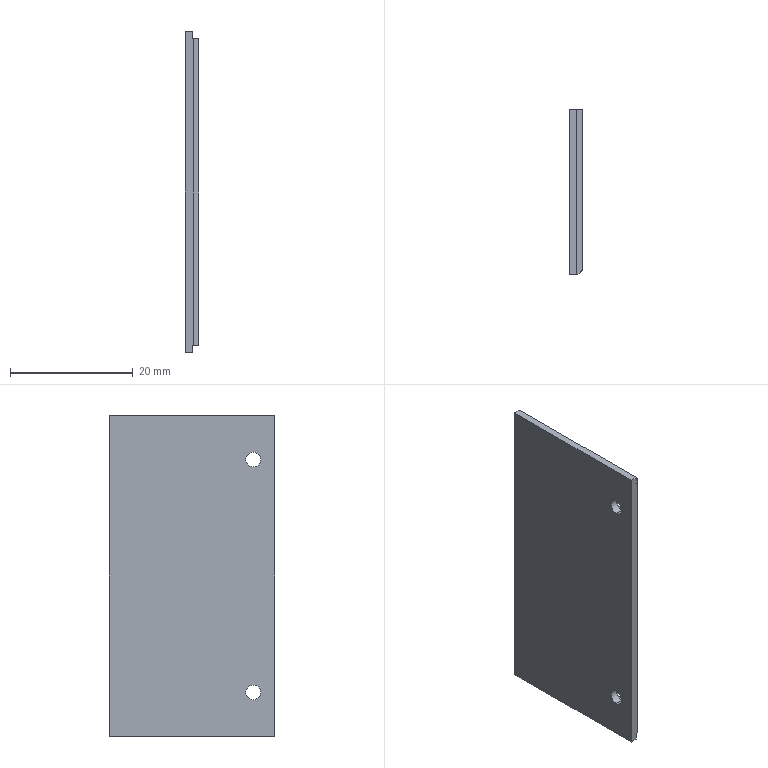Part | STEP file | ASND-0110-OPT-CO60-X-V1.0 lower cover plate | 1 solid | 19 faces | box 2.2 x 27 x 52.3 mm | volume 2996 mm3 | plane 11 | cone 4 | cylinder 4 | commonest cylinder face diameters 2.4 x4
STEP:
#1=CARTESIAN_POINT('',(0.,0.,0.));
#2=DIRECTION('',(0.,0.,1.));
#3=DIRECTION('',(1.,0.,0.));
#4=AXIS2_PLACEMENT_3D('',#1,#2,#3);
#5=CARTESIAN_POINT('',(1.2,-10.,17.8));
#6=VERTEX_POINT('',#5);
#7=CARTESIAN_POINT('',(2.2,-10.,16.8));
#8=VERTEX_POINT('',#7);
#9=CARTESIAN_POINT('',(1.2,-10.,17.8));
#10=DIRECTION('',(0.7071,0.,-0.7071));
#11=VECTOR('',#10,1.);
#12=LINE('',#9,#11);
#13=CARTESIAN_POINT('',(1.2,-10.,19.));
#14=DIRECTION('',(1.,0.,0.));
#15=DIRECTION('',(0.,0.,-1.));
#16=AXIS2_PLACEMENT_3D('',#13,#14,#15);
#17=CONICAL_SURFACE('',#16,1.2,0.7854);
#18=CARTESIAN_POINT('',(6.283,0.));
#19=DIRECTION('',(0.,1.));
#20=VECTOR('',#19,1.);
#21=LINE('',#18,#20);
#22=(GEOMETRIC_REPRESENTATION_CONTEXT(2)PARAMETRIC_REPRESENTATION_CONTEXT()REPRESENTATION_CONTEXT('',''));
#23=DEFINITIONAL_REPRESENTATION('',(#21),#22);
#24=PCURVE('',#17,#23);
#25=CARTESIAN_POINT('',(1.2,-10.,19.));
#26=DIRECTION('',(1.,0.,0.));
#27=DIRECTION('',(0.,0.,-1.));
#28=AXIS2_PLACEMENT_3D('',#25,#26,#27);
#29=CONICAL_SURFACE('',#28,1.2,0.7854);
#30=CARTESIAN_POINT('',(0.,0.));
#31=DIRECTION('',(0.,1.));
#32=VECTOR('',#31,1.);
#33=LINE('',#30,#32);
#34=(GEOMETRIC_REPRESENTATION_CONTEXT(2)PARAMETRIC_REPRESENTATION_CONTEXT()REPRESENTATION_CONTEXT('',''));
#35=DEFINITIONAL_REPRESENTATION('',(#33),#34);
#36=PCURVE('',#29,#35);
#37=SURFACE_CURVE('',#12,(#24,#36),.PCURVE_S1.);
#38=EDGE_CURVE('',#6,#8,#37,.T.);
#39=ORIENTED_EDGE('',*,*,#38,.T.);
#40=CARTESIAN_POINT('',(2.2,-10.,21.2));
#41=VERTEX_POINT('',#40);
#42=CARTESIAN_POINT('',(2.2,-10.,19.));
#43=DIRECTION('',(1.,0.,0.));
#44=DIRECTION('',(0.,0.,-1.));
#45=AXIS2_PLACEMENT_3D('',#42,#43,#44);
#46=CIRCLE('',#45,2.2);
#47=CARTESIAN_POINT('',(0.,1.));
#48=DIRECTION('',(1.,0.));
#49=VECTOR('',#48,1.);
#50=LINE('',#47,#49);
#51=(GEOMETRIC_REPRESENTATION_CONTEXT(2)PARAMETRIC_REPRESENTATION_CONTEXT()REPRESENTATION_CONTEXT('',''));
#52=DEFINITIONAL_REPRESENTATION('',(#50),#51);
#53=PCURVE('',#17,#52);
#54=CARTESIAN_POINT('',(2.2,-12.7,25.));
#55=DIRECTION('',(1.,0.,0.));
#56=DIRECTION('',(0.,0.7071,0.7071));
#57=AXIS2_PLACEMENT_3D('',#54,#55,#56);
#58=PLANE('',#57);
#59=CARTESIAN_POINT('',(-2.333,-6.152));
#60=DIRECTION('',(-0.7071,-0.7071));
#61=AXIS2_PLACEMENT_2D('',#59,#60);
#62=CIRCLE('',#61,2.2);
#63=(GEOMETRIC_REPRESENTATION_CONTEXT(2)PARAMETRIC_REPRESENTATION_CONTEXT()REPRESENTATION_CONTEXT('',''));
#64=DEFINITIONAL_REPRESENTATION('',(#62),#63);
#65=PCURVE('',#58,#64);
#66=SURFACE_CURVE('',#46,(#53,#65),.PCURVE_S1.);
#67=EDGE_CURVE('',#41,#8,#66,.T.);
#68=ORIENTED_EDGE('',*,*,#67,.F.);
#69=CARTESIAN_POINT('',(1.2,-10.,20.2));
#70=VERTEX_POINT('',#69);
#71=CARTESIAN_POINT('',(1.2,-10.,20.2));
#72=DIRECTION('',(0.7071,0.,0.7071));
#73=VECTOR('',#72,1.);
#74=LINE('',#71,#73);
#75=CARTESIAN_POINT('',(3.142,0.));
#76=DIRECTION('',(0.,1.));
#77=VECTOR('',#76,1.);
#78=LINE('',#75,#77);
#79=(GEOMETRIC_REPRESENTATION_CONTEXT(2)PARAMETRIC_REPRESENTATION_CONTEXT()REPRESENTATION_CONTEXT('',''));
#80=DEFINITIONAL_REPRESENTATION('',(#78),#79);
#81=PCURVE('',#17,#80);
#82=CARTESIAN_POINT('',(3.142,0.));
#83=DIRECTION('',(0.,1.));
#84=VECTOR('',#83,1.);
#85=LINE('',#82,#84);
#86=(GEOMETRIC_REPRESENTATION_CONTEXT(2)PARAMETRIC_REPRESENTATION_CONTEXT()REPRESENTATION_CONTEXT('',''));
#87=DEFINITIONAL_REPRESENTATION('',(#85),#86);
#88=PCURVE('',#29,#87);
#89=SURFACE_CURVE('',#74,(#81,#88),.PCURVE_S1.);
#90=EDGE_CURVE('',#70,#41,#89,.T.);
#91=ORIENTED_EDGE('',*,*,#90,.F.);
#92=CARTESIAN_POINT('',(1.2,-10.,19.));
#93=DIRECTION('',(-1.,0.,0.));
#94=DIRECTION('',(0.,0.,-1.));
#95=AXIS2_PLACEMENT_3D('',#92,#93,#94);
#96=CIRCLE('',#95,1.2);
#97=CARTESIAN_POINT('',(6.283,0.));
#98=DIRECTION('',(-1.,0.));
#99=VECTOR('',#98,1.);
#100=LINE('',#97,#99);
#101=(GEOMETRIC_REPRESENTATION_CONTEXT(2)PARAMETRIC_REPRESENTATION_CONTEXT()REPRESENTATION_CONTEXT('',''));
#102=DEFINITIONAL_REPRESENTATION('',(#100),#101);
#103=PCURVE('',#17,#102);
#104=CARTESIAN_POINT('',(0.,-10.,19.));
#105=DIRECTION('',(1.,0.,0.));
#106=DIRECTION('',(0.,0.,-1.));
#107=AXIS2_PLACEMENT_3D('',#104,#105,#106);
#108=CYLINDRICAL_SURFACE('',#107,1.2);
#109=CARTESIAN_POINT('',(6.283,1.2));
#110=DIRECTION('',(-1.,0.));
#111=VECTOR('',#110,1.);
#112=LINE('',#109,#111);
#113=(GEOMETRIC_REPRESENTATION_CONTEXT(2)PARAMETRIC_REPRESENTATION_CONTEXT()REPRESENTATION_CONTEXT('',''));
#114=DEFINITIONAL_REPRESENTATION('',(#112),#113);
#115=PCURVE('',#108,#114);
#116=SURFACE_CURVE('',#96,(#103,#115),.PCURVE_S1.);
#117=EDGE_CURVE('',#6,#70,#116,.T.);
#118=ORIENTED_EDGE('',*,*,#117,.F.);
#119=EDGE_LOOP('',(#39,#68,#91,#118));
#120=FACE_BOUND('',#119,.F.);
#121=ADVANCED_FACE('',(#120),#17,.F.);
#122=CARTESIAN_POINT('',(0.,-10.,17.8));
#123=VERTEX_POINT('',#122);
#124=CARTESIAN_POINT('',(0.,-10.,17.8));
#125=DIRECTION('',(1.,0.,0.));
#126=VECTOR('',#125,1.);
#127=LINE('',#124,#126);
#128=CARTESIAN_POINT('',(6.283,0.));
#129=DIRECTION('',(0.,1.));
#130=VECTOR('',#129,1.);
#131=LINE('',#128,#130);
#132=(GEOMETRIC_REPRESENTATION_CONTEXT(2)PARAMETRIC_REPRESENTATION_CONTEXT()REPRESENTATION_CONTEXT('',''));
#133=DEFINITIONAL_REPRESENTATION('',(#131),#132);
#134=PCURVE('',#108,#133);
#135=CARTESIAN_POINT('',(0.,-10.,19.));
#136=DIRECTION('',(1.,0.,0.));
#137=DIRECTION('',(0.,0.,-1.));
#138=AXIS2_PLACEMENT_3D('',#135,#136,#137);
#139=CYLINDRICAL_SURFACE('',#138,1.2);
#140=CARTESIAN_POINT('',(0.,0.));
#141=DIRECTION('',(0.,1.));
#142=VECTOR('',#141,1.);
#143=LINE('',#140,#142);
#144=(GEOMETRIC_REPRESENTATION_CONTEXT(2)PARAMETRIC_REPRESENTATION_CONTEXT()REPRESENTATION_CONTEXT('',''));
#145=DEFINITIONAL_REPRESENTATION('',(#143),#144);
#146=PCURVE('',#139,#145);
#147=SURFACE_CURVE('',#127,(#134,#146),.PCURVE_S1.);
#148=EDGE_CURVE('',#123,#6,#147,.T.);
#149=ORIENTED_EDGE('',*,*,#148,.T.);
#150=ORIENTED_EDGE('',*,*,#117,.T.);
#151=CARTESIAN_POINT('',(0.,-10.,20.2));
#152=VERTEX_POINT('',#151);
#153=CARTESIAN_POINT('',(0.,-10.,20.2));
#154=DIRECTION('',(1.,0.,0.));
#155=VECTOR('',#154,1.);
#156=LINE('',#153,#155);
#157=CARTESIAN_POINT('',(3.142,0.));
#158=DIRECTION('',(0.,1.));
#159=VECTOR('',#158,1.);
#160=LINE('',#157,#159);
#161=(GEOMETRIC_REPRESENTATION_CONTEXT(2)PARAMETRIC_REPRESENTATION_CONTEXT()REPRESENTATION_CONTEXT('',''));
#162=DEFINITIONAL_REPRESENTATION('',(#160),#161);
#163=PCURVE('',#108,#162);
#164=CARTESIAN_POINT('',(3.142,0.));
#165=DIRECTION('',(0.,1.));
#166=VECTOR('',#165,1.);
#167=LINE('',#164,#166);
#168=(GEOMETRIC_REPRESENTATION_CONTEXT(2)PARAMETRIC_REPRESENTATION_CONTEXT()REPRESENTATION_CONTEXT('',''));
#169=DEFINITIONAL_REPRESENTATION('',(#167),#168);
#170=PCURVE('',#139,#169);
#171=SURFACE_CURVE('',#156,(#163,#170),.PCURVE_S1.);
#172=EDGE_CURVE('',#152,#70,#171,.T.);
#173=ORIENTED_EDGE('',*,*,#172,.F.);
#174=CARTESIAN_POINT('',(0.,-10.,19.));
#175=DIRECTION('',(-1.,0.,0.));
#176=DIRECTION('',(0.,0.,-1.));
#177=AXIS2_PLACEMENT_3D('',#174,#175,#176);
#178=CIRCLE('',#177,1.2);
#179=CARTESIAN_POINT('',(6.283,0.));
#180=DIRECTION('',(-1.,0.));
#181=VECTOR('',#180,1.);
#182=LINE('',#179,#181);
#183=(GEOMETRIC_REPRESENTATION_CONTEXT(2)PARAMETRIC_REPRESENTATION_CONTEXT()REPRESENTATION_CONTEXT('',''));
#184=DEFINITIONAL_REPRESENTATION('',(#182),#183);
#185=PCURVE('',#108,#184);
#186=CARTESIAN_POINT('',(0.,-13.5,26.15));
#187=DIRECTION('',(1.,0.,0.));
#188=DIRECTION('',(0.,0.7071,0.7071));
#189=AXIS2_PLACEMENT_3D('',#186,#187,#188);
#190=PLANE('',#189);
#191=CARTESIAN_POINT('',(-3.429,-8.379));
#192=CARTESIAN_POINT('',(-4.899,-6.91));
#193=CARTESIAN_POINT('',(-2.892,-6.372));
#194=CARTESIAN_POINT('',(-0.8839,-5.834));
#195=CARTESIAN_POINT('',(-1.422,-7.841));
#196=CARTESIAN_POINT('',(-1.96,-9.849));
#197=CARTESIAN_POINT('',(-3.429,-8.379));
#198=(BOUNDED_CURVE()B_SPLINE_CURVE(2,(#191,#192,#193,#194,#195,#196,#197),.UNSPECIFIED.,.T.,.F.)B_SPLINE_CURVE_WITH_KNOTS((1,2,2,2,2,1),(-2.094,0.,2.094,4.189,6.283,8.378),.UNSPECIFIED.)CURVE()GEOMETRIC_REPRESENTATION_ITEM()RATIONAL_B_SPLINE_CURVE((1.,0.5,1.,0.5,1.,0.5,1.))REPRESENTATION_ITEM(''));
#199=(GEOMETRIC_REPRESENTATION_CONTEXT(2)PARAMETRIC_REPRESENTATION_CONTEXT()REPRESENTATION_CONTEXT('',''));
#200=DEFINITIONAL_REPRESENTATION('',(#198),#199);
#201=PCURVE('',#190,#200);
#202=SURFACE_CURVE('',#178,(#185,#201),.PCURVE_S1.);
#203=EDGE_CURVE('',#123,#152,#202,.T.);
#204=ORIENTED_EDGE('',*,*,#203,.F.);
#205=EDGE_LOOP('',(#149,#150,#173,#204));
#206=FACE_BOUND('',#205,.F.);
#207=ADVANCED_FACE('',(#206),#108,.F.);
#208=CARTESIAN_POINT('',(1.2,-10.,-20.2));
#209=VERTEX_POINT('',#208);
#210=CARTESIAN_POINT('',(2.2,-10.,-21.2));
#211=VERTEX_POINT('',#210);
#212=CARTESIAN_POINT('',(1.2,-10.,-20.2));
#213=DIRECTION('',(0.7071,0.,-0.7071));
#214=VECTOR('',#213,1.);
#215=LINE('',#212,#214);
#216=CARTESIAN_POINT('',(1.2,-10.,-19.));
#217=DIRECTION('',(1.,0.,0.));
#218=DIRECTION('',(0.,0.,-1.));
#219=AXIS2_PLACEMENT_3D('',#216,#217,#218);
#220=CONICAL_SURFACE('',#219,1.2,0.7854);
#221=CARTESIAN_POINT('',(6.283,0.));
#222=DIRECTION('',(0.,1.));
#223=VECTOR('',#222,1.);
#224=LINE('',#221,#223);
#225=(GEOMETRIC_REPRESENTATION_CONTEXT(2)PARAMETRIC_REPRESENTATION_CONTEXT()REPRESENTATION_CONTEXT('',''));
#226=DEFINITIONAL_REPRESENTATION('',(#224),#225);
#227=PCURVE('',#220,#226);
#228=CARTESIAN_POINT('',(1.2,-10.,-19.));
#229=DIRECTION('',(1.,0.,0.));
#230=DIRECTION('',(0.,0.,-1.));
#231=AXIS2_PLACEMENT_3D('',#228,#229,#230);
#232=CONICAL_SURFACE('',#231,1.2,0.7854);
#233=CARTESIAN_POINT('',(0.,0.));
#234=DIRECTION('',(0.,1.));
#235=VECTOR('',#234,1.);
#236=LINE('',#233,#235);
#237=(GEOMETRIC_REPRESENTATION_CONTEXT(2)PARAMETRIC_REPRESENTATION_CONTEXT()REPRESENTATION_CONTEXT('',''));
#238=DEFINITIONAL_REPRESENTATION('',(#236),#237);
#239=PCURVE('',#232,#238);
#240=SURFACE_CURVE('',#215,(#227,#239),.PCURVE_S1.);
#241=EDGE_CURVE('',#209,#211,#240,.T.);
#242=ORIENTED_EDGE('',*,*,#241,.T.);
#243=CARTESIAN_POINT('',(2.2,-10.,-16.8));
#244=VERTEX_POINT('',#243);
#245=CARTESIAN_POINT('',(2.2,-10.,-19.));
#246=DIRECTION('',(-1.,0.,0.));
#247=DIRECTION('',(0.,0.,-1.));
#248=AXIS2_PLACEMENT_3D('',#245,#246,#247);
#249=CIRCLE('',#248,2.2);
#250=CARTESIAN_POINT('',(6.283,1.));
#251=DIRECTION('',(-1.,0.));
#252=VECTOR('',#251,1.);
#253=LINE('',#250,#252);
#254=(GEOMETRIC_REPRESENTATION_CONTEXT(2)PARAMETRIC_REPRESENTATION_CONTEXT()REPRESENTATION_CONTEXT('',''));
#255=DEFINITIONAL_REPRESENTATION('',(#253),#254);
#256=PCURVE('',#220,#255);
#257=CARTESIAN_POINT('',(-30.759,-34.578));
#258=CARTESIAN_POINT('',(-33.454,-31.883));
#259=CARTESIAN_POINT('',(-29.773,-30.897));
#260=CARTESIAN_POINT('',(-26.092,-29.911));
#261=CARTESIAN_POINT('',(-27.078,-33.591));
#262=CARTESIAN_POINT('',(-28.065,-37.272));
#263=CARTESIAN_POINT('',(-30.759,-34.578));
#264=(BOUNDED_CURVE()B_SPLINE_CURVE(2,(#257,#258,#259,#260,#261,#262,#263),.UNSPECIFIED.,.T.,.F.)B_SPLINE_CURVE_WITH_KNOTS((1,2,2,2,2,1),(-2.094,0.,2.094,4.189,6.283,8.378),.UNSPECIFIED.)CURVE()GEOMETRIC_REPRESENTATION_ITEM()RATIONAL_B_SPLINE_CURVE((1.,0.5,1.,0.5,1.,0.5,1.))REPRESENTATION_ITEM(''));
#265=(GEOMETRIC_REPRESENTATION_CONTEXT(2)PARAMETRIC_REPRESENTATION_CONTEXT()REPRESENTATION_CONTEXT('',''));
#266=DEFINITIONAL_REPRESENTATION('',(#264),#265);
#267=PCURVE('',#58,#266);
#268=SURFACE_CURVE('',#249,(#256,#267),.PCURVE_S1.);
#269=EDGE_CURVE('',#211,#244,#268,.T.);
#270=ORIENTED_EDGE('',*,*,#269,.T.);
#271=CARTESIAN_POINT('',(1.2,-10.,-17.8));
#272=VERTEX_POINT('',#271);
#273=CARTESIAN_POINT('',(1.2,-10.,-17.8));
#274=DIRECTION('',(0.7071,0.,0.7071));
#275=VECTOR('',#274,1.);
#276=LINE('',#273,#275);
#277=CARTESIAN_POINT('',(3.142,0.));
#278=DIRECTION('',(0.,1.));
#279=VECTOR('',#278,1.);
#280=LINE('',#277,#279);
#281=(GEOMETRIC_REPRESENTATION_CONTEXT(2)PARAMETRIC_REPRESENTATION_CONTEXT()REPRESENTATION_CONTEXT('',''));
#282=DEFINITIONAL_REPRESENTATION('',(#280),#281);
#283=PCURVE('',#220,#282);
#284=CARTESIAN_POINT('',(3.142,0.));
#285=DIRECTION('',(0.,1.));
#286=VECTOR('',#285,1.);
#287=LINE('',#284,#286);
#288=(GEOMETRIC_REPRESENTATION_CONTEXT(2)PARAMETRIC_REPRESENTATION_CONTEXT()REPRESENTATION_CONTEXT('',''));
#289=DEFINITIONAL_REPRESENTATION('',(#287),#288);
#290=PCURVE('',#232,#289);
#291=SURFACE_CURVE('',#276,(#283,#290),.PCURVE_S1.);
#292=EDGE_CURVE('',#272,#244,#291,.T.);
#293=ORIENTED_EDGE('',*,*,#292,.F.);
#294=CARTESIAN_POINT('',(1.2,-10.,-19.));
#295=DIRECTION('',(-1.,0.,0.));
#296=DIRECTION('',(0.,0.,-1.));
#297=AXIS2_PLACEMENT_3D('',#294,#295,#296);
#298=CIRCLE('',#297,1.2);
#299=CARTESIAN_POINT('',(6.283,0.));
#300=DIRECTION('',(-1.,0.));
#301=VECTOR('',#300,1.);
#302=LINE('',#299,#301);
#303=(GEOMETRIC_REPRESENTATION_CONTEXT(2)PARAMETRIC_REPRESENTATION_CONTEXT()REPRESENTATION_CONTEXT('',''));
#304=DEFINITIONAL_REPRESENTATION('',(#302),#303);
#305=PCURVE('',#220,#304);
#306=CARTESIAN_POINT('',(0.,-10.,-19.));
#307=DIRECTION('',(1.,0.,0.));
#308=DIRECTION('',(0.,0.,-1.));
#309=AXIS2_PLACEMENT_3D('',#306,#307,#308);
#310=CYLINDRICAL_SURFACE('',#309,1.2);
#311=CARTESIAN_POINT('',(6.283,1.2));
#312=DIRECTION('',(-1.,0.));
#313=VECTOR('',#312,1.);
#314=LINE('',#311,#313);
#315=(GEOMETRIC_REPRESENTATION_CONTEXT(2)PARAMETRIC_REPRESENTATION_CONTEXT()REPRESENTATION_CONTEXT('',''));
#316=DEFINITIONAL_REPRESENTATION('',(#314),#315);
#317=PCURVE('',#310,#316);
#318=SURFACE_CURVE('',#298,(#305,#317),.PCURVE_S1.);
#319=EDGE_CURVE('',#209,#272,#318,.T.);
#320=ORIENTED_EDGE('',*,*,#319,.F.);
#321=EDGE_LOOP('',(#242,#270,#293,#320));
#322=FACE_BOUND('',#321,.F.);
#323=ADVANCED_FACE('',(#322),#220,.F.);
#324=CARTESIAN_POINT('',(0.,-10.,-20.2));
#325=VERTEX_POINT('',#324);
#326=CARTESIAN_POINT('',(0.,-10.,-20.2));
#327=DIRECTION('',(1.,0.,0.));
#328=VECTOR('',#327,1.);
#329=LINE('',#326,#328);
#330=CARTESIAN_POINT('',(6.283,0.));
#331=DIRECTION('',(0.,1.));
#332=VECTOR('',#331,1.);
#333=LINE('',#330,#332);
#334=(GEOMETRIC_REPRESENTATION_CONTEXT(2)PARAMETRIC_REPRESENTATION_CONTEXT()REPRESENTATION_CONTEXT('',''));
#335=DEFINITIONAL_REPRESENTATION('',(#333),#334);
#336=PCURVE('',#310,#335);
#337=CARTESIAN_POINT('',(0.,-10.,-19.));
#338=DIRECTION('',(1.,0.,0.));
#339=DIRECTION('',(0.,0.,-1.));
#340=AXIS2_PLACEMENT_3D('',#337,#338,#339);
#341=CYLINDRICAL_SURFACE('',#340,1.2);
#342=CARTESIAN_POINT('',(0.,0.));
#343=DIRECTION('',(0.,1.));
#344=VECTOR('',#343,1.);
#345=LINE('',#342,#344);
#346=(GEOMETRIC_REPRESENTATION_CONTEXT(2)PARAMETRIC_REPRESENTATION_CONTEXT()REPRESENTATION_CONTEXT('',''));
#347=DEFINITIONAL_REPRESENTATION('',(#345),#346);
#348=PCURVE('',#341,#347);
#349=SURFACE_CURVE('',#329,(#336,#348),.PCURVE_S1.);
#350=EDGE_CURVE('',#325,#209,#349,.T.);
#351=ORIENTED_EDGE('',*,*,#350,.T.);
#352=ORIENTED_EDGE('',*,*,#319,.T.);
#353=CARTESIAN_POINT('',(0.,-10.,-17.8));
#354=VERTEX_POINT('',#353);
#355=CARTESIAN_POINT('',(0.,-10.,-17.8));
#356=DIRECTION('',(1.,0.,0.));
#357=VECTOR('',#356,1.);
#358=LINE('',#355,#357);
#359=CARTESIAN_POINT('',(3.142,0.));
#360=DIRECTION('',(0.,1.));
#361=VECTOR('',#360,1.);
#362=LINE('',#359,#361);
#363=(GEOMETRIC_REPRESENTATION_CONTEXT(2)PARAMETRIC_REPRESENTATION_CONTEXT()REPRESENTATION_CONTEXT('',''));
#364=DEFINITIONAL_REPRESENTATION('',(#362),#363);
#365=PCURVE('',#310,#364);
#366=CARTESIAN_POINT('',(3.142,0.));
#367=DIRECTION('',(0.,1.));
#368=VECTOR('',#367,1.);
#369=LINE('',#366,#368);
#370=(GEOMETRIC_REPRESENTATION_CONTEXT(2)PARAMETRIC_REPRESENTATION_CONTEXT()REPRESENTATION_CONTEXT('',''));
#371=DEFINITIONAL_REPRESENTATION('',(#369),#370);
#372=PCURVE('',#341,#371);
#373=SURFACE_CURVE('',#358,(#365,#372),.PCURVE_S1.);
#374=EDGE_CURVE('',#354,#272,#373,.T.);
#375=ORIENTED_EDGE('',*,*,#374,.F.);
#376=CARTESIAN_POINT('',(0.,-10.,-19.));
#377=DIRECTION('',(-1.,0.,0.));
#378=DIRECTION('',(0.,0.,-1.));
#379=AXIS2_PLACEMENT_3D('',#376,#377,#378);
#380=CIRCLE('',#379,1.2);
#381=CARTESIAN_POINT('',(6.283,0.));
#382=DIRECTION('',(-1.,0.));
#383=VECTOR('',#382,1.);
#384=LINE('',#381,#383);
#385=(GEOMETRIC_REPRESENTATION_CONTEXT(2)PARAMETRIC_REPRESENTATION_CONTEXT()REPRESENTATION_CONTEXT('',''));
#386=DEFINITIONAL_REPRESENTATION('',(#384),#385);
#387=PCURVE('',#310,#386);
#388=CARTESIAN_POINT('',(-30.3,-35.249));
#389=CARTESIAN_POINT('',(-31.769,-33.78));
#390=CARTESIAN_POINT('',(-29.762,-33.242));
#391=CARTESIAN_POINT('',(-27.754,-32.704));
#392=CARTESIAN_POINT('',(-28.292,-34.711));
#393=CARTESIAN_POINT('',(-28.83,-36.719));
#394=CARTESIAN_POINT('',(-30.3,-35.249));
#395=(BOUNDED_CURVE()B_SPLINE_CURVE(2,(#388,#389,#390,#391,#392,#393,#394),.UNSPECIFIED.,.T.,.F.)B_SPLINE_CURVE_WITH_KNOTS((1,2,2,2,2,1),(-2.094,0.,2.094,4.189,6.283,8.378),.UNSPECIFIED.)CURVE()GEOMETRIC_REPRESENTATION_ITEM()RATIONAL_B_SPLINE_CURVE((1.,0.5,1.,0.5,1.,0.5,1.))REPRESENTATION_ITEM(''));
#396=(GEOMETRIC_REPRESENTATION_CONTEXT(2)PARAMETRIC_REPRESENTATION_CONTEXT()REPRESENTATION_CONTEXT('',''));
#397=DEFINITIONAL_REPRESENTATION('',(#395),#396);
#398=PCURVE('',#190,#397);
#399=SURFACE_CURVE('',#380,(#387,#398),.PCURVE_S1.);
#400=EDGE_CURVE('',#325,#354,#399,.T.);
#401=ORIENTED_EDGE('',*,*,#400,.F.);
#402=EDGE_LOOP('',(#351,#352,#375,#401));
#403=FACE_BOUND('',#402,.F.);
#404=ADVANCED_FACE('',(#403),#310,.F.);
#405=CARTESIAN_POINT('',(1.15,-13.5,-26.15));
#406=VERTEX_POINT('',#405);
#407=CARTESIAN_POINT('',(0.,-13.5,-26.15));
#408=VERTEX_POINT('',#407);
#409=CARTESIAN_POINT('',(1.15,-13.5,-26.15));
#410=DIRECTION('',(-1.,0.,0.));
#411=VECTOR('',#410,1.);
#412=LINE('',#409,#411);
#413=CARTESIAN_POINT('',(0.,-13.5,-26.15));
#414=DIRECTION('',(0.,0.,1.));
#415=DIRECTION('',(0.7071,0.7071,0.));
#416=AXIS2_PLACEMENT_3D('',#413,#414,#415);
#417=PLANE('',#416);
#418=CARTESIAN_POINT('',(0.8132,-0.8132));
#419=DIRECTION('',(-0.7071,0.7071));
#420=VECTOR('',#419,1.);
#421=LINE('',#418,#420);
#422=(GEOMETRIC_REPRESENTATION_CONTEXT(2)PARAMETRIC_REPRESENTATION_CONTEXT()REPRESENTATION_CONTEXT('',''));
#423=DEFINITIONAL_REPRESENTATION('',(#421),#422);
#424=PCURVE('',#417,#423);
#425=CARTESIAN_POINT('',(0.,-13.5,-26.15));
#426=DIRECTION('',(0.,1.,0.));
#427=DIRECTION('',(0.7071,0.,0.7071));
#428=AXIS2_PLACEMENT_3D('',#425,#426,#427);
#429=PLANE('',#428);
#430=CARTESIAN_POINT('',(0.8132,0.8132));
#431=DIRECTION('',(-0.7071,-0.7071));
#432=VECTOR('',#431,1.);
#433=LINE('',#430,#432);
#434=(GEOMETRIC_REPRESENTATION_CONTEXT(2)PARAMETRIC_REPRESENTATION_CONTEXT()REPRESENTATION_CONTEXT('',''));
#435=DEFINITIONAL_REPRESENTATION('',(#433),#434);
#436=PCURVE('',#429,#435);
#437=SURFACE_CURVE('',#412,(#424,#436),.PCURVE_S1.);
#438=EDGE_CURVE('',#406,#408,#437,.T.);
#439=ORIENTED_EDGE('',*,*,#438,.T.);
#440=CARTESIAN_POINT('',(0.,13.5,-26.15));
#441=VERTEX_POINT('',#440);
#442=CARTESIAN_POINT('',(0.,-13.5,-26.15));
#443=DIRECTION('',(0.,1.,0.));
#444=VECTOR('',#443,1.);
#445=LINE('',#442,#444);
#446=CARTESIAN_POINT('',(0.,0.));
#447=DIRECTION('',(0.7071,0.7071));
#448=VECTOR('',#447,1.);
#449=LINE('',#446,#448);
#450=(GEOMETRIC_REPRESENTATION_CONTEXT(2)PARAMETRIC_REPRESENTATION_CONTEXT()REPRESENTATION_CONTEXT('',''));
#451=DEFINITIONAL_REPRESENTATION('',(#449),#450);
#452=PCURVE('',#417,#451);
#453=CARTESIAN_POINT('',(-36.982,-36.982));
#454=DIRECTION('',(0.7071,-0.7071));
#455=VECTOR('',#454,1.);
#456=LINE('',#453,#455);
#457=(GEOMETRIC_REPRESENTATION_CONTEXT(2)PARAMETRIC_REPRESENTATION_CONTEXT()REPRESENTATION_CONTEXT('',''));
#458=DEFINITIONAL_REPRESENTATION('',(#456),#457);
#459=PCURVE('',#190,#458);
#460=SURFACE_CURVE('',#445,(#452,#459),.PCURVE_S1.);
#461=EDGE_CURVE('',#408,#441,#460,.T.);
#462=ORIENTED_EDGE('',*,*,#461,.T.);
#463=CARTESIAN_POINT('',(1.15,13.5,-26.15));
#464=VERTEX_POINT('',#463);
#465=CARTESIAN_POINT('',(1.15,13.5,-26.15));
#466=DIRECTION('',(-1.,0.,0.));
#467=VECTOR('',#466,1.);
#468=LINE('',#465,#467);
#469=CARTESIAN_POINT('',(19.905,18.279));
#470=DIRECTION('',(-0.7071,0.7071));
#471=VECTOR('',#470,1.);
#472=LINE('',#469,#471);
#473=(GEOMETRIC_REPRESENTATION_CONTEXT(2)PARAMETRIC_REPRESENTATION_CONTEXT()REPRESENTATION_CONTEXT('',''));
#474=DEFINITIONAL_REPRESENTATION('',(#472),#473);
#475=PCURVE('',#417,#474);
#476=CARTESIAN_POINT('',(0.,13.5,26.15));
#477=DIRECTION('',(0.,-1.,0.));
#478=DIRECTION('',(0.7071,0.,0.7071));
#479=AXIS2_PLACEMENT_3D('',#476,#477,#478);
#480=PLANE('',#479);
#481=CARTESIAN_POINT('',(-36.169,-37.795));
#482=DIRECTION('',(-0.7071,0.7071));
#483=VECTOR('',#482,1.);
#484=LINE('',#481,#483);
#485=(GEOMETRIC_REPRESENTATION_CONTEXT(2)PARAMETRIC_REPRESENTATION_CONTEXT()REPRESENTATION_CONTEXT('',''));
#486=DEFINITIONAL_REPRESENTATION('',(#484),#485);
#487=PCURVE('',#480,#486);
#488=SURFACE_CURVE('',#468,(#475,#487),.PCURVE_S1.);
#489=EDGE_CURVE('',#464,#441,#488,.T.);
#490=ORIENTED_EDGE('',*,*,#489,.F.);
#491=CARTESIAN_POINT('',(1.15,-13.5,-26.15));
#492=DIRECTION('',(0.,1.,0.));
#493=VECTOR('',#492,1.);
#494=LINE('',#491,#493);
#495=CARTESIAN_POINT('',(0.8132,-0.8132));
#496=DIRECTION('',(0.7071,0.7071));
#497=VECTOR('',#496,1.);
#498=LINE('',#495,#497);
#499=(GEOMETRIC_REPRESENTATION_CONTEXT(2)PARAMETRIC_REPRESENTATION_CONTEXT()REPRESENTATION_CONTEXT('',''));
#500=DEFINITIONAL_REPRESENTATION('',(#498),#499);
#501=PCURVE('',#417,#500);
#502=CARTESIAN_POINT('',(1.15,-13.5,-25.));
#503=DIRECTION('',(1.,0.,0.));
#504=DIRECTION('',(0.,0.7071,0.7071));
#505=AXIS2_PLACEMENT_3D('',#502,#503,#504);
#506=PLANE('',#505);
#507=CARTESIAN_POINT('',(-0.8132,-0.8132));
#508=DIRECTION('',(0.7071,-0.7071));
#509=VECTOR('',#508,1.);
#510=LINE('',#507,#509);
#511=(GEOMETRIC_REPRESENTATION_CONTEXT(2)PARAMETRIC_REPRESENTATION_CONTEXT()REPRESENTATION_CONTEXT('',''));
#512=DEFINITIONAL_REPRESENTATION('',(#510),#511);
#513=PCURVE('',#506,#512);
#514=SURFACE_CURVE('',#494,(#501,#513),.PCURVE_S1.);
#515=EDGE_CURVE('',#406,#464,#514,.T.);
#516=ORIENTED_EDGE('',*,*,#515,.F.);
#517=EDGE_LOOP('',(#439,#462,#490,#516));
#518=FACE_BOUND('',#517,.T.);
#519=ADVANCED_FACE('',(#518),#417,.F.);
#520=CARTESIAN_POINT('',(0.,13.5,26.15));
#521=VERTEX_POINT('',#520);
#522=CARTESIAN_POINT('',(1.15,13.5,26.15));
#523=VERTEX_POINT('',#522);
#524=CARTESIAN_POINT('',(0.,13.5,26.15));
#525=DIRECTION('',(1.,0.,0.));
#526=VECTOR('',#525,1.);
#527=LINE('',#524,#526);
#528=CARTESIAN_POINT('',(1.15,-13.5,26.15));
#529=DIRECTION('',(0.,0.,-1.));
#530=DIRECTION('',(0.7071,0.7071,0.));
#531=AXIS2_PLACEMENT_3D('',#528,#529,#530);
#532=PLANE('',#531);
#533=CARTESIAN_POINT('',(18.279,-19.905));
#534=DIRECTION('',(0.7071,0.7071));
#535=VECTOR('',#534,1.);
#536=LINE('',#533,#535);
#537=(GEOMETRIC_REPRESENTATION_CONTEXT(2)PARAMETRIC_REPRESENTATION_CONTEXT()REPRESENTATION_CONTEXT('',''));
#538=DEFINITIONAL_REPRESENTATION('',(#536),#537);
#539=PCURVE('',#532,#538);
#540=CARTESIAN_POINT('',(0.,0.));
#541=DIRECTION('',(0.7071,-0.7071));
#542=VECTOR('',#541,1.);
#543=LINE('',#540,#542);
#544=(GEOMETRIC_REPRESENTATION_CONTEXT(2)PARAMETRIC_REPRESENTATION_CONTEXT()REPRESENTATION_CONTEXT('',''));
#545=DEFINITIONAL_REPRESENTATION('',(#543),#544);
#546=PCURVE('',#480,#545);
#547=SURFACE_CURVE('',#527,(#539,#546),.PCURVE_S1.);
#548=EDGE_CURVE('',#521,#523,#547,.T.);
#549=ORIENTED_EDGE('',*,*,#548,.F.);
#550=CARTESIAN_POINT('',(0.,-13.5,26.15));
#551=VERTEX_POINT('',#550);
#552=CARTESIAN_POINT('',(0.,13.5,26.15));
#553=DIRECTION('',(0.,-1.,0.));
#554=VECTOR('',#553,1.);
#555=LINE('',#552,#554);
#556=CARTESIAN_POINT('',(18.279,-19.905));
#557=DIRECTION('',(-0.7071,0.7071));
#558=VECTOR('',#557,1.);
#559=LINE('',#556,#558);
#560=(GEOMETRIC_REPRESENTATION_CONTEXT(2)PARAMETRIC_REPRESENTATION_CONTEXT()REPRESENTATION_CONTEXT('',''));
#561=DEFINITIONAL_REPRESENTATION('',(#559),#560);
#562=PCURVE('',#532,#561);
#563=CARTESIAN_POINT('',(19.092,-19.092));
#564=DIRECTION('',(-0.7071,0.7071));
#565=VECTOR('',#564,1.);
#566=LINE('',#563,#565);
#567=(GEOMETRIC_REPRESENTATION_CONTEXT(2)PARAMETRIC_REPRESENTATION_CONTEXT()REPRESENTATION_CONTEXT('',''));
#568=DEFINITIONAL_REPRESENTATION('',(#566),#567);
#569=PCURVE('',#190,#568);
#570=SURFACE_CURVE('',#555,(#562,#569),.PCURVE_S1.);
#571=EDGE_CURVE('',#521,#551,#570,.T.);
#572=ORIENTED_EDGE('',*,*,#571,.T.);
#573=CARTESIAN_POINT('',(1.15,-13.5,26.15));
#574=VERTEX_POINT('',#573);
#575=CARTESIAN_POINT('',(0.,-13.5,26.15));
#576=DIRECTION('',(1.,0.,0.));
#577=VECTOR('',#576,1.);
#578=LINE('',#575,#577);
#579=CARTESIAN_POINT('',(-0.8132,-0.8132));
#580=DIRECTION('',(0.7071,0.7071));
#581=VECTOR('',#580,1.);
#582=LINE('',#579,#581);
#583=(GEOMETRIC_REPRESENTATION_CONTEXT(2)PARAMETRIC_REPRESENTATION_CONTEXT()REPRESENTATION_CONTEXT('',''));
#584=DEFINITIONAL_REPRESENTATION('',(#582),#583);
#585=PCURVE('',#532,#584);
#586=CARTESIAN_POINT('',(36.982,-36.982));
#587=DIRECTION('',(0.7071,0.7071));
#588=VECTOR('',#587,1.);
#589=LINE('',#586,#588);
#590=(GEOMETRIC_REPRESENTATION_CONTEXT(2)PARAMETRIC_REPRESENTATION_CONTEXT()REPRESENTATION_CONTEXT('',''));
#591=DEFINITIONAL_REPRESENTATION('',(#589),#590);
#592=PCURVE('',#429,#591);
#593=SURFACE_CURVE('',#578,(#585,#592),.PCURVE_S1.);
#594=EDGE_CURVE('',#551,#574,#593,.T.);
#595=ORIENTED_EDGE('',*,*,#594,.T.);
#596=CARTESIAN_POINT('',(1.15,13.5,26.15));
#597=DIRECTION('',(0.,-1.,0.));
#598=VECTOR('',#597,1.);
#599=LINE('',#596,#598);
#600=CARTESIAN_POINT('',(19.092,-19.092));
#601=DIRECTION('',(-0.7071,0.7071));
#602=VECTOR('',#601,1.);
#603=LINE('',#600,#602);
#604=(GEOMETRIC_REPRESENTATION_CONTEXT(2)PARAMETRIC_REPRESENTATION_CONTEXT()REPRESENTATION_CONTEXT('',''));
#605=DEFINITIONAL_REPRESENTATION('',(#603),#604);
#606=PCURVE('',#532,#605);
#607=CARTESIAN_POINT('',(1.15,-13.5,26.15));
#608=DIRECTION('',(1.,0.,0.));
#609=DIRECTION('',(0.,0.7071,0.7071));
#610=AXIS2_PLACEMENT_3D('',#607,#608,#609);
#611=PLANE('',#610);
#612=CARTESIAN_POINT('',(19.092,-19.092));
#613=DIRECTION('',(-0.7071,0.7071));
#614=VECTOR('',#613,1.);
#615=LINE('',#612,#614);
#616=(GEOMETRIC_REPRESENTATION_CONTEXT(2)PARAMETRIC_REPRESENTATION_CONTEXT()REPRESENTATION_CONTEXT('',''));
#617=DEFINITIONAL_REPRESENTATION('',(#615),#616);
#618=PCURVE('',#611,#617);
#619=SURFACE_CURVE('',#599,(#606,#618),.PCURVE_S1.);
#620=EDGE_CURVE('',#523,#574,#619,.T.);
#621=ORIENTED_EDGE('',*,*,#620,.F.);
#622=EDGE_LOOP('',(#549,#572,#595,#621));
#623=FACE_BOUND('',#622,.T.);
#624=ADVANCED_FACE('',(#623),#532,.F.);
#625=CARTESIAN_POINT('',(1.15,13.5,25.));
#626=VERTEX_POINT('',#625);
#627=CARTESIAN_POINT('',(1.15,13.5,25.));
#628=DIRECTION('',(0.,0.,1.));
#629=VECTOR('',#628,1.);
#630=LINE('',#627,#629);
#631=CARTESIAN_POINT('',(18.279,-19.905));
#632=DIRECTION('',(0.7071,0.7071));
#633=VECTOR('',#632,1.);
#634=LINE('',#631,#633);
#635=(GEOMETRIC_REPRESENTATION_CONTEXT(2)PARAMETRIC_REPRESENTATION_CONTEXT()REPRESENTATION_CONTEXT('',''));
#636=DEFINITIONAL_REPRESENTATION('',(#634),#635);
#637=PCURVE('',#611,#636);
#638=CARTESIAN_POINT('',(-0.000000003,-1.626));
#639=DIRECTION('',(0.7071,0.7071));
#640=VECTOR('',#639,1.);
#641=LINE('',#638,#640);
#642=(GEOMETRIC_REPRESENTATION_CONTEXT(2)PARAMETRIC_REPRESENTATION_CONTEXT()REPRESENTATION_CONTEXT('',''));
#643=DEFINITIONAL_REPRESENTATION('',(#641),#642);
#644=PCURVE('',#480,#643);
#645=SURFACE_CURVE('',#630,(#637,#644),.PCURVE_S1.);
#646=EDGE_CURVE('',#626,#523,#645,.T.);
#647=ORIENTED_EDGE('',*,*,#646,.T.);
#648=ORIENTED_EDGE('',*,*,#620,.T.);
#649=CARTESIAN_POINT('',(1.15,-13.5,25.));
#650=VERTEX_POINT('',#649);
#651=CARTESIAN_POINT('',(1.15,-13.5,26.15));
#652=DIRECTION('',(0.,0.,-1.));
#653=VECTOR('',#652,1.);
#654=LINE('',#651,#653);
#655=CARTESIAN_POINT('',(0.,0.));
#656=DIRECTION('',(-0.7071,-0.7071));
#657=VECTOR('',#656,1.);
#658=LINE('',#655,#657);
#659=(GEOMETRIC_REPRESENTATION_CONTEXT(2)PARAMETRIC_REPRESENTATION_CONTEXT()REPRESENTATION_CONTEXT('',''));
#660=DEFINITIONAL_REPRESENTATION('',(#658),#659);
#661=PCURVE('',#611,#660);
#662=CARTESIAN_POINT('',(37.795,-36.169));
#663=DIRECTION('',(-0.7071,0.7071));
#664=VECTOR('',#663,1.);
#665=LINE('',#662,#664);
#666=(GEOMETRIC_REPRESENTATION_CONTEXT(2)PARAMETRIC_REPRESENTATION_CONTEXT()REPRESENTATION_CONTEXT('',''));
#667=DEFINITIONAL_REPRESENTATION('',(#665),#666);
#668=PCURVE('',#429,#667);
#669=SURFACE_CURVE('',#654,(#661,#668),.PCURVE_S1.);
#670=EDGE_CURVE('',#574,#650,#669,.T.);
#671=ORIENTED_EDGE('',*,*,#670,.T.);
#672=CARTESIAN_POINT('',(1.15,-13.5,25.));
#673=DIRECTION('',(0.,1.,0.));
#674=VECTOR('',#673,1.);
#675=LINE('',#672,#674);
#676=CARTESIAN_POINT('',(-0.8132,-0.8132));
#677=DIRECTION('',(0.7071,-0.7071));
#678=VECTOR('',#677,1.);
#679=LINE('',#676,#678);
#680=(GEOMETRIC_REPRESENTATION_CONTEXT(2)PARAMETRIC_REPRESENTATION_CONTEXT()REPRESENTATION_CONTEXT('',''));
#681=DEFINITIONAL_REPRESENTATION('',(#679),#680);
#682=PCURVE('',#611,#681);
#683=CARTESIAN_POINT('',(1.15,-13.5,25.));
#684=DIRECTION('',(0.,0.,-1.));
#685=DIRECTION('',(0.7071,0.7071,0.));
#686=AXIS2_PLACEMENT_3D('',#683,#684,#685);
#687=PLANE('',#686);
#688=CARTESIAN_POINT('',(0.,0.));
#689=DIRECTION('',(0.7071,-0.7071));
#690=VECTOR('',#689,1.);
#691=LINE('',#688,#690);
#692=(GEOMETRIC_REPRESENTATION_CONTEXT(2)PARAMETRIC_REPRESENTATION_CONTEXT()REPRESENTATION_CONTEXT('',''));
#693=DEFINITIONAL_REPRESENTATION('',(#691),#692);
#694=PCURVE('',#687,#693);
#695=SURFACE_CURVE('',#675,(#682,#694),.PCURVE_S1.);
#696=EDGE_CURVE('',#650,#626,#695,.T.);
#697=ORIENTED_EDGE('',*,*,#696,.T.);
#698=EDGE_LOOP('',(#647,#648,#671,#697));
#699=FACE_BOUND('',#698,.T.);
#700=ADVANCED_FACE('',(#699),#611,.T.);
#701=CARTESIAN_POINT('',(1.4,-13.5,25.));
#702=VERTEX_POINT('',#701);
#703=CARTESIAN_POINT('',(1.4,-13.5,-25.));
#704=VERTEX_POINT('',#703);
#705=CARTESIAN_POINT('',(1.4,-13.5,25.));
#706=DIRECTION('',(0.,0.,-1.));
#707=VECTOR('',#706,1.);
#708=LINE('',#705,#707);
#709=CARTESIAN_POINT('',(37.158,-35.179));
#710=DIRECTION('',(-0.7071,0.7071));
#711=VECTOR('',#710,1.);
#712=LINE('',#709,#711);
#713=(GEOMETRIC_REPRESENTATION_CONTEXT(2)PARAMETRIC_REPRESENTATION_CONTEXT()REPRESENTATION_CONTEXT('',''));
#714=DEFINITIONAL_REPRESENTATION('',(#712),#713);
#715=PCURVE('',#429,#714);
#716=CARTESIAN_POINT('',(1.4,-13.5,-25.));
#717=DIRECTION('',(0.7071,-0.7071,0.));
#718=DIRECTION('',(0.5774,0.5774,0.5774));
#719=AXIS2_PLACEMENT_3D('',#716,#717,#718);
#720=PLANE('',#719);
#721=CARTESIAN_POINT('',(28.868,40.825));
#722=DIRECTION('',(-0.5774,-0.8165));
#723=VECTOR('',#722,1.);
#724=LINE('',#721,#723);
#725=(GEOMETRIC_REPRESENTATION_CONTEXT(2)PARAMETRIC_REPRESENTATION_CONTEXT()REPRESENTATION_CONTEXT('',''));
#726=DEFINITIONAL_REPRESENTATION('',(#724),#725);
#727=PCURVE('',#720,#726);
#728=SURFACE_CURVE('',#708,(#715,#727),.PCURVE_S1.);
#729=EDGE_CURVE('',#702,#704,#728,.T.);
#730=ORIENTED_EDGE('',*,*,#729,.F.);
#731=CARTESIAN_POINT('',(1.4,-13.5,25.));
#732=DIRECTION('',(-1.,0.,0.));
#733=VECTOR('',#732,1.);
#734=LINE('',#731,#733);
#735=CARTESIAN_POINT('',(37.158,-35.179));
#736=DIRECTION('',(-0.7071,-0.7071));
#737=VECTOR('',#736,1.);
#738=LINE('',#735,#737);
#739=(GEOMETRIC_REPRESENTATION_CONTEXT(2)PARAMETRIC_REPRESENTATION_CONTEXT()REPRESENTATION_CONTEXT('',''));
#740=DEFINITIONAL_REPRESENTATION('',(#738),#739);
#741=PCURVE('',#429,#740);
#742=CARTESIAN_POINT('',(0.1768,0.1768));
#743=DIRECTION('',(-0.7071,-0.7071));
#744=VECTOR('',#743,1.);
#745=LINE('',#742,#744);
#746=(GEOMETRIC_REPRESENTATION_CONTEXT(2)PARAMETRIC_REPRESENTATION_CONTEXT()REPRESENTATION_CONTEXT('',''));
#747=DEFINITIONAL_REPRESENTATION('',(#745),#746);
#748=PCURVE('',#687,#747);
#749=SURFACE_CURVE('',#734,(#741,#748),.PCURVE_S1.);
#750=EDGE_CURVE('',#702,#650,#749,.T.);
#751=ORIENTED_EDGE('',*,*,#750,.T.);
#752=ORIENTED_EDGE('',*,*,#670,.F.);
#753=ORIENTED_EDGE('',*,*,#594,.F.);
#754=CARTESIAN_POINT('',(0.,-13.5,26.15));
#755=DIRECTION('',(0.,0.,-1.));
#756=VECTOR('',#755,1.);
#757=LINE('',#754,#756);
#758=CARTESIAN_POINT('',(36.982,-36.982));
#759=DIRECTION('',(-0.7071,0.7071));
#760=VECTOR('',#759,1.);
#761=LINE('',#758,#760);
#762=(GEOMETRIC_REPRESENTATION_CONTEXT(2)PARAMETRIC_REPRESENTATION_CONTEXT()REPRESENTATION_CONTEXT('',''));
#763=DEFINITIONAL_REPRESENTATION('',(#761),#762);
#764=PCURVE('',#429,#763);
#765=CARTESIAN_POINT('',(0.,0.));
#766=DIRECTION('',(-0.7071,-0.7071));
#767=VECTOR('',#766,1.);
#768=LINE('',#765,#767);
#769=(GEOMETRIC_REPRESENTATION_CONTEXT(2)PARAMETRIC_REPRESENTATION_CONTEXT()REPRESENTATION_CONTEXT('',''));
#770=DEFINITIONAL_REPRESENTATION('',(#768),#769);
#771=PCURVE('',#190,#770);
#772=SURFACE_CURVE('',#757,(#764,#771),.PCURVE_S1.);
#773=EDGE_CURVE('',#551,#408,#772,.T.);
#774=ORIENTED_EDGE('',*,*,#773,.T.);
#775=ORIENTED_EDGE('',*,*,#438,.F.);
#776=CARTESIAN_POINT('',(1.15,-13.5,-25.));
#777=VERTEX_POINT('',#776);
#778=CARTESIAN_POINT('',(1.15,-13.5,-25.));
#779=DIRECTION('',(0.,0.,-1.));
#780=VECTOR('',#779,1.);
#781=LINE('',#778,#780);
#782=CARTESIAN_POINT('',(1.626,-0.000000005));
#783=DIRECTION('',(-0.7071,0.7071));
#784=VECTOR('',#783,1.);
#785=LINE('',#782,#784);
#786=(GEOMETRIC_REPRESENTATION_CONTEXT(2)PARAMETRIC_REPRESENTATION_CONTEXT()REPRESENTATION_CONTEXT('',''));
#787=DEFINITIONAL_REPRESENTATION('',(#785),#786);
#788=PCURVE('',#429,#787);
#789=CARTESIAN_POINT('',(0.000000005,0.000000005));
#790=DIRECTION('',(-0.7071,-0.7071));
#791=VECTOR('',#790,1.);
#792=LINE('',#789,#791);
#793=(GEOMETRIC_REPRESENTATION_CONTEXT(2)PARAMETRIC_REPRESENTATION_CONTEXT()REPRESENTATION_CONTEXT('',''));
#794=DEFINITIONAL_REPRESENTATION('',(#792),#793);
#795=PCURVE('',#506,#794);
#796=SURFACE_CURVE('',#781,(#788,#795),.PCURVE_S1.);
#797=EDGE_CURVE('',#777,#406,#796,.T.);
#798=ORIENTED_EDGE('',*,*,#797,.F.);
#799=CARTESIAN_POINT('',(1.4,-13.5,-25.));
#800=DIRECTION('',(-1.,0.,0.));
#801=VECTOR('',#800,1.);
#802=LINE('',#799,#801);
#803=CARTESIAN_POINT('',(1.803,0.1768));
#804=DIRECTION('',(-0.7071,-0.7071));
#805=VECTOR('',#804,1.);
#806=LINE('',#803,#805);
#807=(GEOMETRIC_REPRESENTATION_CONTEXT(2)PARAMETRIC_REPRESENTATION_CONTEXT()REPRESENTATION_CONTEXT('',''));
#808=DEFINITIONAL_REPRESENTATION('',(#806),#807);
#809=PCURVE('',#429,#808);
#810=CARTESIAN_POINT('',(1.15,13.5,-25.));
#811=DIRECTION('',(0.,0.,1.));
#812=DIRECTION('',(0.7071,0.7071,0.));
#813=AXIS2_PLACEMENT_3D('',#810,#811,#812);
#814=PLANE('',#813);
#815=CARTESIAN_POINT('',(-18.915,-19.269));
#816=DIRECTION('',(-0.7071,0.7071));
#817=VECTOR('',#816,1.);
#818=LINE('',#815,#817);
#819=(GEOMETRIC_REPRESENTATION_CONTEXT(2)PARAMETRIC_REPRESENTATION_CONTEXT()REPRESENTATION_CONTEXT('',''));
#820=DEFINITIONAL_REPRESENTATION('',(#818),#819);
#821=PCURVE('',#814,#820);
#822=SURFACE_CURVE('',#802,(#809,#821),.PCURVE_S1.);
#823=EDGE_CURVE('',#704,#777,#822,.T.);
#824=ORIENTED_EDGE('',*,*,#823,.F.);
#825=EDGE_LOOP('',(#730,#751,#752,#753,#774,#775,#798,#824));
#826=FACE_BOUND('',#825,.T.);
#827=ADVANCED_FACE('',(#826),#429,.F.);
#828=CARTESIAN_POINT('',(1.15,13.5,-25.));
#829=VERTEX_POINT('',#828);
#830=CARTESIAN_POINT('',(1.15,13.5,-26.15));
#831=DIRECTION('',(0.,0.,1.));
#832=VECTOR('',#831,1.);
#833=LINE('',#830,#832);
#834=CARTESIAN_POINT('',(18.279,-19.905));
#835=DIRECTION('',(0.7071,0.7071));
#836=VECTOR('',#835,1.);
#837=LINE('',#834,#836);
#838=(GEOMETRIC_REPRESENTATION_CONTEXT(2)PARAMETRIC_REPRESENTATION_CONTEXT()REPRESENTATION_CONTEXT('',''));
#839=DEFINITIONAL_REPRESENTATION('',(#837),#838);
#840=PCURVE('',#506,#839);
#841=CARTESIAN_POINT('',(-36.169,-37.795));
#842=DIRECTION('',(0.7071,0.7071));
#843=VECTOR('',#842,1.);
#844=LINE('',#841,#843);
#845=(GEOMETRIC_REPRESENTATION_CONTEXT(2)PARAMETRIC_REPRESENTATION_CONTEXT()REPRESENTATION_CONTEXT('',''));
#846=DEFINITIONAL_REPRESENTATION('',(#844),#845);
#847=PCURVE('',#480,#846);
#848=SURFACE_CURVE('',#833,(#840,#847),.PCURVE_S1.);
#849=EDGE_CURVE('',#464,#829,#848,.T.);
#850=ORIENTED_EDGE('',*,*,#849,.T.);
#851=CARTESIAN_POINT('',(1.15,13.5,-25.));
#852=DIRECTION('',(0.,-1.,0.));
#853=VECTOR('',#852,1.);
#854=LINE('',#851,#853);
#855=CARTESIAN_POINT('',(19.092,-19.092));
#856=DIRECTION('',(-0.7071,0.7071));
#857=VECTOR('',#856,1.);
#858=LINE('',#855,#857);
#859=(GEOMETRIC_REPRESENTATION_CONTEXT(2)PARAMETRIC_REPRESENTATION_CONTEXT()REPRESENTATION_CONTEXT('',''));
#860=DEFINITIONAL_REPRESENTATION('',(#858),#859);
#861=PCURVE('',#506,#860);
#862=CARTESIAN_POINT('',(0.,0.));
#863=DIRECTION('',(-0.7071,-0.7071));
#864=VECTOR('',#863,1.);
#865=LINE('',#862,#864);
#866=(GEOMETRIC_REPRESENTATION_CONTEXT(2)PARAMETRIC_REPRESENTATION_CONTEXT()REPRESENTATION_CONTEXT('',''));
#867=DEFINITIONAL_REPRESENTATION('',(#865),#866);
#868=PCURVE('',#814,#867);
#869=SURFACE_CURVE('',#854,(#861,#868),.PCURVE_S1.);
#870=EDGE_CURVE('',#829,#777,#869,.T.);
#871=ORIENTED_EDGE('',*,*,#870,.T.);
#872=ORIENTED_EDGE('',*,*,#797,.T.);
#873=ORIENTED_EDGE('',*,*,#515,.T.);
#874=EDGE_LOOP('',(#850,#871,#872,#873));
#875=FACE_BOUND('',#874,.T.);
#876=ADVANCED_FACE('',(#875),#506,.T.);
#877=CARTESIAN_POINT('',(1.2,-10.,-19.));
#878=DIRECTION('',(-1.,0.,0.));
#879=DIRECTION('',(0.,0.,-1.));
#880=AXIS2_PLACEMENT_3D('',#877,#878,#879);
#881=CIRCLE('',#880,1.2);
#882=CARTESIAN_POINT('',(6.283,1.2));
#883=DIRECTION('',(-1.,0.));
#884=VECTOR('',#883,1.);
#885=LINE('',#882,#884);
#886=(GEOMETRIC_REPRESENTATION_CONTEXT(2)PARAMETRIC_REPRESENTATION_CONTEXT()REPRESENTATION_CONTEXT('',''));
#887=DEFINITIONAL_REPRESENTATION('',(#885),#886);
#888=PCURVE('',#341,#887);
#889=CARTESIAN_POINT('',(6.283,0.));
#890=DIRECTION('',(-1.,0.));
#891=VECTOR('',#890,1.);
#892=LINE('',#889,#891);
#893=(GEOMETRIC_REPRESENTATION_CONTEXT(2)PARAMETRIC_REPRESENTATION_CONTEXT()REPRESENTATION_CONTEXT('',''));
#894=DEFINITIONAL_REPRESENTATION('',(#892),#893);
#895=PCURVE('',#232,#894);
#896=SURFACE_CURVE('',#881,(#888,#895),.PCURVE_S1.);
#897=EDGE_CURVE('',#272,#209,#896,.T.);
#898=ORIENTED_EDGE('',*,*,#897,.T.);
#899=ORIENTED_EDGE('',*,*,#350,.F.);
#900=CARTESIAN_POINT('',(0.,-10.,-19.));
#901=DIRECTION('',(-1.,0.,0.));
#902=DIRECTION('',(0.,0.,-1.));
#903=AXIS2_PLACEMENT_3D('',#900,#901,#902);
#904=CIRCLE('',#903,1.2);
#905=CARTESIAN_POINT('',(6.283,0.));
#906=DIRECTION('',(-1.,0.));
#907=VECTOR('',#906,1.);
#908=LINE('',#905,#907);
#909=(GEOMETRIC_REPRESENTATION_CONTEXT(2)PARAMETRIC_REPRESENTATION_CONTEXT()REPRESENTATION_CONTEXT('',''));
#910=DEFINITIONAL_REPRESENTATION('',(#908),#909);
#911=PCURVE('',#341,#910);
#912=CARTESIAN_POINT('',(-30.3,-35.249));
#913=CARTESIAN_POINT('',(-31.769,-33.78));
#914=CARTESIAN_POINT('',(-29.762,-33.242));
#915=CARTESIAN_POINT('',(-27.754,-32.704));
#916=CARTESIAN_POINT('',(-28.292,-34.711));
#917=CARTESIAN_POINT('',(-28.83,-36.719));
#918=CARTESIAN_POINT('',(-30.3,-35.249));
#919=(BOUNDED_CURVE()B_SPLINE_CURVE(2,(#912,#913,#914,#915,#916,#917,#918),.UNSPECIFIED.,.T.,.F.)B_SPLINE_CURVE_WITH_KNOTS((1,2,2,2,2,1),(-2.094,0.,2.094,4.189,6.283,8.378),.UNSPECIFIED.)CURVE()GEOMETRIC_REPRESENTATION_ITEM()RATIONAL_B_SPLINE_CURVE((1.,0.5,1.,0.5,1.,0.5,1.))REPRESENTATION_ITEM(''));
#920=(GEOMETRIC_REPRESENTATION_CONTEXT(2)PARAMETRIC_REPRESENTATION_CONTEXT()REPRESENTATION_CONTEXT('',''));
#921=DEFINITIONAL_REPRESENTATION('',(#919),#920);
#922=PCURVE('',#190,#921);
#923=SURFACE_CURVE('',#904,(#911,#922),.PCURVE_S1.);
#924=EDGE_CURVE('',#354,#325,#923,.T.);
#925=ORIENTED_EDGE('',*,*,#924,.F.);
#926=ORIENTED_EDGE('',*,*,#374,.T.);
#927=EDGE_LOOP('',(#898,#899,#925,#926));
#928=FACE_BOUND('',#927,.F.);
#929=ADVANCED_FACE('',(#928),#341,.F.);
#930=CARTESIAN_POINT('',(0.,13.5,26.15));
#931=DIRECTION('',(0.,0.,-1.));
#932=VECTOR('',#931,1.);
#933=LINE('',#930,#932);
#934=CARTESIAN_POINT('',(19.092,-19.092));
#935=DIRECTION('',(-0.7071,-0.7071));
#936=VECTOR('',#935,1.);
#937=LINE('',#934,#936);
#938=(GEOMETRIC_REPRESENTATION_CONTEXT(2)PARAMETRIC_REPRESENTATION_CONTEXT()REPRESENTATION_CONTEXT('',''));
#939=DEFINITIONAL_REPRESENTATION('',(#937),#938);
#940=PCURVE('',#190,#939);
#941=CARTESIAN_POINT('',(0.,0.));
#942=DIRECTION('',(-0.7071,-0.7071));
#943=VECTOR('',#942,1.);
#944=LINE('',#941,#943);
#945=(GEOMETRIC_REPRESENTATION_CONTEXT(2)PARAMETRIC_REPRESENTATION_CONTEXT()REPRESENTATION_CONTEXT('',''));
#946=DEFINITIONAL_REPRESENTATION('',(#944),#945);
#947=PCURVE('',#480,#946);
#948=SURFACE_CURVE('',#933,(#940,#947),.PCURVE_S1.);
#949=EDGE_CURVE('',#521,#441,#948,.T.);
#950=ORIENTED_EDGE('',*,*,#949,.T.);
#951=ORIENTED_EDGE('',*,*,#461,.F.);
#952=ORIENTED_EDGE('',*,*,#773,.F.);
#953=ORIENTED_EDGE('',*,*,#571,.F.);
#954=EDGE_LOOP('',(#950,#951,#952,#953));
#955=FACE_BOUND('',#954,.T.);
#956=ORIENTED_EDGE('',*,*,#400,.F.);
#957=ORIENTED_EDGE('',*,*,#924,.F.);
#958=EDGE_LOOP('',(#956,#957));
#959=FACE_BOUND('',#958,.T.);
#960=ORIENTED_EDGE('',*,*,#203,.F.);
#961=CARTESIAN_POINT('',(0.,-10.,19.));
#962=DIRECTION('',(-1.,0.,0.));
#963=DIRECTION('',(0.,0.,-1.));
#964=AXIS2_PLACEMENT_3D('',#961,#962,#963);
#965=CIRCLE('',#964,1.2);
#966=CARTESIAN_POINT('',(-3.429,-8.379));
#967=CARTESIAN_POINT('',(-4.899,-6.91));
#968=CARTESIAN_POINT('',(-2.892,-6.372));
#969=CARTESIAN_POINT('',(-0.8839,-5.834));
#970=CARTESIAN_POINT('',(-1.422,-7.841));
#971=CARTESIAN_POINT('',(-1.96,-9.849));
#972=CARTESIAN_POINT('',(-3.429,-8.379));
#973=(BOUNDED_CURVE()B_SPLINE_CURVE(2,(#966,#967,#968,#969,#970,#971,#972),.UNSPECIFIED.,.T.,.F.)B_SPLINE_CURVE_WITH_KNOTS((1,2,2,2,2,1),(-2.094,0.,2.094,4.189,6.283,8.378),.UNSPECIFIED.)CURVE()GEOMETRIC_REPRESENTATION_ITEM()RATIONAL_B_SPLINE_CURVE((1.,0.5,1.,0.5,1.,0.5,1.))REPRESENTATION_ITEM(''));
#974=(GEOMETRIC_REPRESENTATION_CONTEXT(2)PARAMETRIC_REPRESENTATION_CONTEXT()REPRESENTATION_CONTEXT('',''));
#975=DEFINITIONAL_REPRESENTATION('',(#973),#974);
#976=PCURVE('',#190,#975);
#977=CARTESIAN_POINT('',(6.283,0.));
#978=DIRECTION('',(-1.,0.));
#979=VECTOR('',#978,1.);
#980=LINE('',#977,#979);
#981=(GEOMETRIC_REPRESENTATION_CONTEXT(2)PARAMETRIC_REPRESENTATION_CONTEXT()REPRESENTATION_CONTEXT('',''));
#982=DEFINITIONAL_REPRESENTATION('',(#980),#981);
#983=PCURVE('',#139,#982);
#984=SURFACE_CURVE('',#965,(#976,#983),.PCURVE_S1.);
#985=EDGE_CURVE('',#152,#123,#984,.T.);
#986=ORIENTED_EDGE('',*,*,#985,.F.);
#987=EDGE_LOOP('',(#960,#986));
#988=FACE_BOUND('',#987,.T.);
#989=ADVANCED_FACE('',(#955,#959,#988),#190,.F.);
#990=CARTESIAN_POINT('',(2.2,-12.7,25.));
#991=VERTEX_POINT('',#990);
#992=CARTESIAN_POINT('',(2.2,-12.7,25.));
#993=DIRECTION('',(-0.7071,-0.7071,0.));
#994=VECTOR('',#993,1.);
#995=LINE('',#992,#994);
#996=CARTESIAN_POINT('',(1.308,0.1768));
#997=DIRECTION('',(-1.,0.));
#998=VECTOR('',#997,1.);
#999=LINE('',#996,#998);
#1000=(GEOMETRIC_REPRESENTATION_CONTEXT(2)PARAMETRIC_REPRESENTATION_CONTEXT()REPRESENTATION_CONTEXT('',''));
#1001=DEFINITIONAL_REPRESENTATION('',(#999),#1000);
#1002=PCURVE('',#687,#1001);
#1003=CARTESIAN_POINT('',(29.791,40.172));
#1004=DIRECTION('',(-0.8165,0.5774));
#1005=VECTOR('',#1004,1.);
#1006=LINE('',#1003,#1005);
#1007=(GEOMETRIC_REPRESENTATION_CONTEXT(2)PARAMETRIC_REPRESENTATION_CONTEXT()REPRESENTATION_CONTEXT('',''));
#1008=DEFINITIONAL_REPRESENTATION('',(#1006),#1007);
#1009=PCURVE('',#720,#1008);
#1010=SURFACE_CURVE('',#995,(#1002,#1009),.PCURVE_S1.);
#1011=EDGE_CURVE('',#991,#702,#1010,.T.);
#1012=ORIENTED_EDGE('',*,*,#1011,.F.);
#1013=CARTESIAN_POINT('',(2.2,13.5,25.));
#1014=VERTEX_POINT('',#1013);
#1015=CARTESIAN_POINT('',(2.2,13.5,25.));
#1016=DIRECTION('',(0.,-1.,0.));
#1017=VECTOR('',#1016,1.);
#1018=LINE('',#1015,#1017);
#1019=CARTESIAN_POINT('',(19.834,-18.349));
#1020=DIRECTION('',(-0.7071,0.7071));
#1021=VECTOR('',#1020,1.);
#1022=LINE('',#1019,#1021);
#1023=(GEOMETRIC_REPRESENTATION_CONTEXT(2)PARAMETRIC_REPRESENTATION_CONTEXT()REPRESENTATION_CONTEXT('',''));
#1024=DEFINITIONAL_REPRESENTATION('',(#1022),#1023);
#1025=PCURVE('',#687,#1024);
#1026=CARTESIAN_POINT('',(18.526,-18.526));
#1027=DIRECTION('',(-0.7071,0.7071));
#1028=VECTOR('',#1027,1.);
#1029=LINE('',#1026,#1028);
#1030=(GEOMETRIC_REPRESENTATION_CONTEXT(2)PARAMETRIC_REPRESENTATION_CONTEXT()REPRESENTATION_CONTEXT('',''));
#1031=DEFINITIONAL_REPRESENTATION('',(#1029),#1030);
#1032=PCURVE('',#58,#1031);
#1033=SURFACE_CURVE('',#1018,(#1025,#1032),.PCURVE_S1.);
#1034=EDGE_CURVE('',#1014,#991,#1033,.T.);
#1035=ORIENTED_EDGE('',*,*,#1034,.F.);
#1036=CARTESIAN_POINT('',(2.2,13.5,25.));
#1037=DIRECTION('',(-1.,0.,0.));
#1038=VECTOR('',#1037,1.);
#1039=LINE('',#1036,#1038);
#1040=CARTESIAN_POINT('',(19.834,-18.349));
#1041=DIRECTION('',(-0.7071,-0.7071));
#1042=VECTOR('',#1041,1.);
#1043=LINE('',#1040,#1042);
#1044=(GEOMETRIC_REPRESENTATION_CONTEXT(2)PARAMETRIC_REPRESENTATION_CONTEXT()REPRESENTATION_CONTEXT('',''));
#1045=DEFINITIONAL_REPRESENTATION('',(#1043),#1044);
#1046=PCURVE('',#687,#1045);
#1047=CARTESIAN_POINT('',(0.7425,-2.369));
#1048=DIRECTION('',(-0.7071,0.7071));
#1049=VECTOR('',#1048,1.);
#1050=LINE('',#1047,#1049);
#1051=(GEOMETRIC_REPRESENTATION_CONTEXT(2)PARAMETRIC_REPRESENTATION_CONTEXT()REPRESENTATION_CONTEXT('',''));
#1052=DEFINITIONAL_REPRESENTATION('',(#1050),#1051);
#1053=PCURVE('',#480,#1052);
#1054=SURFACE_CURVE('',#1039,(#1046,#1053),.PCURVE_S1.);
#1055=EDGE_CURVE('',#1014,#626,#1054,.T.);
#1056=ORIENTED_EDGE('',*,*,#1055,.T.);
#1057=ORIENTED_EDGE('',*,*,#696,.F.);
#1058=ORIENTED_EDGE('',*,*,#750,.F.);
#1059=EDGE_LOOP('',(#1012,#1035,#1056,#1057,#1058));
#1060=FACE_BOUND('',#1059,.T.);
#1061=ADVANCED_FACE('',(#1060),#687,.F.);
#1062=CARTESIAN_POINT('',(2.2,-12.7,-25.));
#1063=VERTEX_POINT('',#1062);
#1064=CARTESIAN_POINT('',(1.4,-13.5,-25.));
#1065=DIRECTION('',(0.7071,0.7071,0.));
#1066=VECTOR('',#1065,1.);
#1067=LINE('',#1064,#1066);
#1068=CARTESIAN_POINT('',(0.000000002,0.000000003));
#1069=DIRECTION('',(0.8165,-0.5774));
#1070=VECTOR('',#1069,1.);
#1071=LINE('',#1068,#1070);
#1072=(GEOMETRIC_REPRESENTATION_CONTEXT(2)PARAMETRIC_REPRESENTATION_CONTEXT()REPRESENTATION_CONTEXT('',''));
#1073=DEFINITIONAL_REPRESENTATION('',(#1071),#1072);
#1074=PCURVE('',#720,#1073);
#1075=CARTESIAN_POINT('',(-18.915,-19.269));
#1076=DIRECTION('',(1.,0.));
#1077=VECTOR('',#1076,1.);
#1078=LINE('',#1075,#1077);
#1079=(GEOMETRIC_REPRESENTATION_CONTEXT(2)PARAMETRIC_REPRESENTATION_CONTEXT()REPRESENTATION_CONTEXT('',''));
#1080=DEFINITIONAL_REPRESENTATION('',(#1078),#1079);
#1081=PCURVE('',#814,#1080);
#1082=SURFACE_CURVE('',#1067,(#1074,#1081),.PCURVE_S1.);
#1083=EDGE_CURVE('',#704,#1063,#1082,.T.);
#1084=ORIENTED_EDGE('',*,*,#1083,.T.);
#1085=CARTESIAN_POINT('',(2.2,-12.7,25.));
#1086=DIRECTION('',(0.,0.,-1.));
#1087=VECTOR('',#1086,1.);
#1088=LINE('',#1085,#1087);
#1089=CARTESIAN_POINT('',(29.791,40.172));
#1090=DIRECTION('',(-0.5774,-0.8165));
#1091=VECTOR('',#1090,1.);
#1092=LINE('',#1089,#1091);
#1093=(GEOMETRIC_REPRESENTATION_CONTEXT(2)PARAMETRIC_REPRESENTATION_CONTEXT()REPRESENTATION_CONTEXT('',''));
#1094=DEFINITIONAL_REPRESENTATION('',(#1092),#1093);
#1095=PCURVE('',#720,#1094);
#1096=CARTESIAN_POINT('',(0.,0.));
#1097=DIRECTION('',(-0.7071,-0.7071));
#1098=VECTOR('',#1097,1.);
#1099=LINE('',#1096,#1098);
#1100=(GEOMETRIC_REPRESENTATION_CONTEXT(2)PARAMETRIC_REPRESENTATION_CONTEXT()REPRESENTATION_CONTEXT('',''));
#1101=DEFINITIONAL_REPRESENTATION('',(#1099),#1100);
#1102=PCURVE('',#58,#1101);
#1103=SURFACE_CURVE('',#1088,(#1095,#1102),.PCURVE_S1.);
#1104=EDGE_CURVE('',#991,#1063,#1103,.T.);
#1105=ORIENTED_EDGE('',*,*,#1104,.F.);
#1106=ORIENTED_EDGE('',*,*,#1011,.T.);
#1107=ORIENTED_EDGE('',*,*,#729,.T.);
#1108=EDGE_LOOP('',(#1084,#1105,#1106,#1107));
#1109=FACE_BOUND('',#1108,.T.);
#1110=ADVANCED_FACE('',(#1109),#720,.T.);
#1111=ORIENTED_EDGE('',*,*,#1083,.F.);
#1112=ORIENTED_EDGE('',*,*,#823,.T.);
#1113=ORIENTED_EDGE('',*,*,#870,.F.);
#1114=CARTESIAN_POINT('',(2.2,13.5,-25.));
#1115=VERTEX_POINT('',#1114);
#1116=CARTESIAN_POINT('',(1.15,13.5,-25.));
#1117=DIRECTION('',(1.,0.,0.));
#1118=VECTOR('',#1117,1.);
#1119=LINE('',#1116,#1118);
#1120=CARTESIAN_POINT('',(0.,0.));
#1121=DIRECTION('',(0.7071,-0.7071));
#1122=VECTOR('',#1121,1.);
#1123=LINE('',#1120,#1122);
#1124=(GEOMETRIC_REPRESENTATION_CONTEXT(2)PARAMETRIC_REPRESENTATION_CONTEXT()REPRESENTATION_CONTEXT('',''));
#1125=DEFINITIONAL_REPRESENTATION('',(#1123),#1124);
#1126=PCURVE('',#814,#1125);
#1127=CARTESIAN_POINT('',(-35.355,-36.982));
#1128=DIRECTION('',(0.7071,-0.7071));
#1129=VECTOR('',#1128,1.);
#1130=LINE('',#1127,#1129);
#1131=(GEOMETRIC_REPRESENTATION_CONTEXT(2)PARAMETRIC_REPRESENTATION_CONTEXT()REPRESENTATION_CONTEXT('',''));
#1132=DEFINITIONAL_REPRESENTATION('',(#1130),#1131);
#1133=PCURVE('',#480,#1132);
#1134=SURFACE_CURVE('',#1119,(#1126,#1133),.PCURVE_S1.);
#1135=EDGE_CURVE('',#829,#1115,#1134,.T.);
#1136=ORIENTED_EDGE('',*,*,#1135,.T.);
#1137=CARTESIAN_POINT('',(2.2,-12.7,-25.));
#1138=DIRECTION('',(0.,1.,0.));
#1139=VECTOR('',#1138,1.);
#1140=LINE('',#1137,#1139);
#1141=CARTESIAN_POINT('',(-17.784,-19.269));
#1142=DIRECTION('',(0.7071,0.7071));
#1143=VECTOR('',#1142,1.);
#1144=LINE('',#1141,#1143);
#1145=(GEOMETRIC_REPRESENTATION_CONTEXT(2)PARAMETRIC_REPRESENTATION_CONTEXT()REPRESENTATION_CONTEXT('',''));
#1146=DEFINITIONAL_REPRESENTATION('',(#1144),#1145);
#1147=PCURVE('',#814,#1146);
#1148=CARTESIAN_POINT('',(-35.355,-35.355));
#1149=DIRECTION('',(0.7071,-0.7071));
#1150=VECTOR('',#1149,1.);
#1151=LINE('',#1148,#1150);
#1152=(GEOMETRIC_REPRESENTATION_CONTEXT(2)PARAMETRIC_REPRESENTATION_CONTEXT()REPRESENTATION_CONTEXT('',''));
#1153=DEFINITIONAL_REPRESENTATION('',(#1151),#1152);
#1154=PCURVE('',#58,#1153);
#1155=SURFACE_CURVE('',#1140,(#1147,#1154),.PCURVE_S1.);
#1156=EDGE_CURVE('',#1063,#1115,#1155,.T.);
#1157=ORIENTED_EDGE('',*,*,#1156,.F.);
#1158=EDGE_LOOP('',(#1111,#1112,#1113,#1136,#1157));
#1159=FACE_BOUND('',#1158,.T.);
#1160=ADVANCED_FACE('',(#1159),#814,.F.);
#1161=ORIENTED_EDGE('',*,*,#1135,.F.);
#1162=ORIENTED_EDGE('',*,*,#849,.F.);
#1163=ORIENTED_EDGE('',*,*,#489,.T.);
#1164=ORIENTED_EDGE('',*,*,#949,.F.);
#1165=ORIENTED_EDGE('',*,*,#548,.T.);
#1166=ORIENTED_EDGE('',*,*,#646,.F.);
#1167=ORIENTED_EDGE('',*,*,#1055,.F.);
#1168=CARTESIAN_POINT('',(2.2,13.5,-25.));
#1169=DIRECTION('',(0.,0.,1.));
#1170=VECTOR('',#1169,1.);
#1171=LINE('',#1168,#1170);
#1172=CARTESIAN_POINT('',(-34.613,-37.724));
#1173=DIRECTION('',(0.7071,0.7071));
#1174=VECTOR('',#1173,1.);
#1175=LINE('',#1172,#1174);
#1176=(GEOMETRIC_REPRESENTATION_CONTEXT(2)PARAMETRIC_REPRESENTATION_CONTEXT()REPRESENTATION_CONTEXT('',''));
#1177=DEFINITIONAL_REPRESENTATION('',(#1175),#1176);
#1178=PCURVE('',#480,#1177);
#1179=CARTESIAN_POINT('',(-16.829,-53.882));
#1180=DIRECTION('',(0.7071,0.7071));
#1181=VECTOR('',#1180,1.);
#1182=LINE('',#1179,#1181);
#1183=(GEOMETRIC_REPRESENTATION_CONTEXT(2)PARAMETRIC_REPRESENTATION_CONTEXT()REPRESENTATION_CONTEXT('',''));
#1184=DEFINITIONAL_REPRESENTATION('',(#1182),#1183);
#1185=PCURVE('',#58,#1184);
#1186=SURFACE_CURVE('',#1171,(#1178,#1185),.PCURVE_S1.);
#1187=EDGE_CURVE('',#1115,#1014,#1186,.T.);
#1188=ORIENTED_EDGE('',*,*,#1187,.F.);
#1189=EDGE_LOOP('',(#1161,#1162,#1163,#1164,#1165,#1166,#1167,#1188));
#1190=FACE_BOUND('',#1189,.T.);
#1191=ADVANCED_FACE('',(#1190),#480,.F.);
#1192=CARTESIAN_POINT('',(2.2,-10.,-19.));
#1193=DIRECTION('',(-1.,0.,0.));
#1194=DIRECTION('',(0.,0.,-1.));
#1195=AXIS2_PLACEMENT_3D('',#1192,#1193,#1194);
#1196=CIRCLE('',#1195,2.2);
#1197=CARTESIAN_POINT('',(6.283,1.));
#1198=DIRECTION('',(-1.,0.));
#1199=VECTOR('',#1198,1.);
#1200=LINE('',#1197,#1199);
#1201=(GEOMETRIC_REPRESENTATION_CONTEXT(2)PARAMETRIC_REPRESENTATION_CONTEXT()REPRESENTATION_CONTEXT('',''));
#1202=DEFINITIONAL_REPRESENTATION('',(#1200),#1201);
#1203=PCURVE('',#232,#1202);
#1204=CARTESIAN_POINT('',(-30.759,-34.578));
#1205=CARTESIAN_POINT('',(-33.454,-31.883));
#1206=CARTESIAN_POINT('',(-29.773,-30.897));
#1207=CARTESIAN_POINT('',(-26.092,-29.911));
#1208=CARTESIAN_POINT('',(-27.078,-33.591));
#1209=CARTESIAN_POINT('',(-28.065,-37.272));
#1210=CARTESIAN_POINT('',(-30.759,-34.578));
#1211=(BOUNDED_CURVE()B_SPLINE_CURVE(2,(#1204,#1205,#1206,#1207,#1208,#1209,#1210),.UNSPECIFIED.,.T.,.F.)B_SPLINE_CURVE_WITH_KNOTS((1,2,2,2,2,1),(-2.094,0.,2.094,4.189,6.283,8.378),.UNSPECIFIED.)CURVE()GEOMETRIC_REPRESENTATION_ITEM()RATIONAL_B_SPLINE_CURVE((1.,0.5,1.,0.5,1.,0.5,1.))REPRESENTATION_ITEM(''));
#1212=(GEOMETRIC_REPRESENTATION_CONTEXT(2)PARAMETRIC_REPRESENTATION_CONTEXT()REPRESENTATION_CONTEXT('',''));
#1213=DEFINITIONAL_REPRESENTATION('',(#1211),#1212);
#1214=PCURVE('',#58,#1213);
#1215=SURFACE_CURVE('',#1196,(#1203,#1214),.PCURVE_S1.);
#1216=EDGE_CURVE('',#244,#211,#1215,.T.);
#1217=ORIENTED_EDGE('',*,*,#1216,.T.);
#1218=ORIENTED_EDGE('',*,*,#241,.F.);
#1219=ORIENTED_EDGE('',*,*,#897,.F.);
#1220=ORIENTED_EDGE('',*,*,#292,.T.);
#1221=EDGE_LOOP('',(#1217,#1218,#1219,#1220));
#1222=FACE_BOUND('',#1221,.F.);
#1223=ADVANCED_FACE('',(#1222),#232,.F.);
#1224=CARTESIAN_POINT('',(1.2,-10.,19.));
#1225=DIRECTION('',(-1.,0.,0.));
#1226=DIRECTION('',(0.,0.,-1.));
#1227=AXIS2_PLACEMENT_3D('',#1224,#1225,#1226);
#1228=CIRCLE('',#1227,1.2);
#1229=CARTESIAN_POINT('',(6.283,1.2));
#1230=DIRECTION('',(-1.,0.));
#1231=VECTOR('',#1230,1.);
#1232=LINE('',#1229,#1231);
#1233=(GEOMETRIC_REPRESENTATION_CONTEXT(2)PARAMETRIC_REPRESENTATION_CONTEXT()REPRESENTATION_CONTEXT('',''));
#1234=DEFINITIONAL_REPRESENTATION('',(#1232),#1233);
#1235=PCURVE('',#139,#1234);
#1236=CARTESIAN_POINT('',(6.283,0.));
#1237=DIRECTION('',(-1.,0.));
#1238=VECTOR('',#1237,1.);
#1239=LINE('',#1236,#1238);
#1240=(GEOMETRIC_REPRESENTATION_CONTEXT(2)PARAMETRIC_REPRESENTATION_CONTEXT()REPRESENTATION_CONTEXT('',''));
#1241=DEFINITIONAL_REPRESENTATION('',(#1239),#1240);
#1242=PCURVE('',#29,#1241);
#1243=SURFACE_CURVE('',#1228,(#1235,#1242),.PCURVE_S1.);
#1244=EDGE_CURVE('',#70,#6,#1243,.T.);
#1245=ORIENTED_EDGE('',*,*,#1244,.T.);
#1246=ORIENTED_EDGE('',*,*,#148,.F.);
#1247=ORIENTED_EDGE('',*,*,#985,.F.);
#1248=ORIENTED_EDGE('',*,*,#172,.T.);
#1249=EDGE_LOOP('',(#1245,#1246,#1247,#1248));
#1250=FACE_BOUND('',#1249,.F.);
#1251=ADVANCED_FACE('',(#1250),#139,.F.);
#1252=ORIENTED_EDGE('',*,*,#1156,.T.);
#1253=ORIENTED_EDGE('',*,*,#1187,.T.);
#1254=ORIENTED_EDGE('',*,*,#1034,.T.);
#1255=ORIENTED_EDGE('',*,*,#1104,.T.);
#1256=EDGE_LOOP('',(#1252,#1253,#1254,#1255));
#1257=FACE_BOUND('',#1256,.T.);
#1258=ORIENTED_EDGE('',*,*,#269,.T.);
#1259=ORIENTED_EDGE('',*,*,#1216,.T.);
#1260=EDGE_LOOP('',(#1258,#1259));
#1261=FACE_BOUND('',#1260,.T.);
#1262=CARTESIAN_POINT('',(2.2,-10.,19.));
#1263=DIRECTION('',(1.,0.,0.));
#1264=DIRECTION('',(0.,0.,-1.));
#1265=AXIS2_PLACEMENT_3D('',#1262,#1263,#1264);
#1266=CIRCLE('',#1265,2.2);
#1267=CARTESIAN_POINT('',(-2.333,-6.152));
#1268=DIRECTION('',(-0.7071,-0.7071));
#1269=AXIS2_PLACEMENT_2D('',#1267,#1268);
#1270=CIRCLE('',#1269,2.2);
#1271=(GEOMETRIC_REPRESENTATION_CONTEXT(2)PARAMETRIC_REPRESENTATION_CONTEXT()REPRESENTATION_CONTEXT('',''));
#1272=DEFINITIONAL_REPRESENTATION('',(#1270),#1271);
#1273=PCURVE('',#58,#1272);
#1274=CARTESIAN_POINT('',(0.,1.));
#1275=DIRECTION('',(1.,0.));
#1276=VECTOR('',#1275,1.);
#1277=LINE('',#1274,#1276);
#1278=(GEOMETRIC_REPRESENTATION_CONTEXT(2)PARAMETRIC_REPRESENTATION_CONTEXT()REPRESENTATION_CONTEXT('',''));
#1279=DEFINITIONAL_REPRESENTATION('',(#1277),#1278);
#1280=PCURVE('',#29,#1279);
#1281=SURFACE_CURVE('',#1266,(#1273,#1280),.PCURVE_S1.);
#1282=EDGE_CURVE('',#8,#41,#1281,.T.);
#1283=ORIENTED_EDGE('',*,*,#1282,.F.);
#1284=ORIENTED_EDGE('',*,*,#67,.F.);
#1285=EDGE_LOOP('',(#1283,#1284));
#1286=FACE_BOUND('',#1285,.T.);
#1287=ADVANCED_FACE('',(#1257,#1261,#1286),#58,.T.);
#1288=ORIENTED_EDGE('',*,*,#1282,.F.);
#1289=ORIENTED_EDGE('',*,*,#38,.F.);
#1290=ORIENTED_EDGE('',*,*,#1244,.F.);
#1291=ORIENTED_EDGE('',*,*,#90,.T.);
#1292=EDGE_LOOP('',(#1288,#1289,#1290,#1291));
#1293=FACE_BOUND('',#1292,.F.);
#1294=ADVANCED_FACE('',(#1293),#29,.F.);
#1295=CLOSED_SHELL('',(#121,#207,#323,#404,#519,#624,#700,#827,#876,#929,#989,#1061,#1110,#1160,#1191,#1223,#1251,#1287,#1294));
#1296=MANIFOLD_SOLID_BREP('',#1295);
#1297=(LENGTH_UNIT()NAMED_UNIT(*)SI_UNIT(.MILLI.,.METRE.));
#1298=UNCERTAINTY_MEASURE_WITH_UNIT(LENGTH_MEASURE(0.0000001),#1297,'','');
#1299=(NAMED_UNIT(*)PLANE_ANGLE_UNIT()SI_UNIT($,.RADIAN.));
#1300=(NAMED_UNIT(*)SI_UNIT($,.STERADIAN.)SOLID_ANGLE_UNIT());
#1301=(GEOMETRIC_REPRESENTATION_CONTEXT(3)GLOBAL_UNCERTAINTY_ASSIGNED_CONTEXT((#1298))GLOBAL_UNIT_ASSIGNED_CONTEXT((#1297,#1299,#1300))REPRESENTATION_CONTEXT('',''));
#1302=ADVANCED_BREP_SHAPE_REPRESENTATION('',(#4,#1296),#1301);